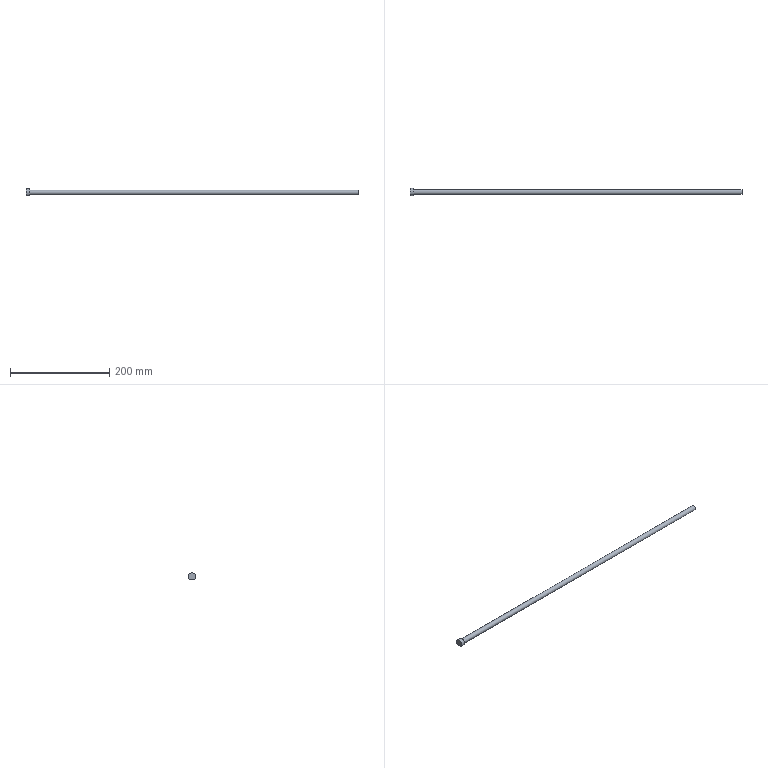Part | STEP file | solid 42 | 1 solid | 6 faces | box 670 x 15 x 13 mm | volume 53295 mm3 | plane 4 | cylinder 2 | commonest cylinder face diameters 10 x1 15 x1